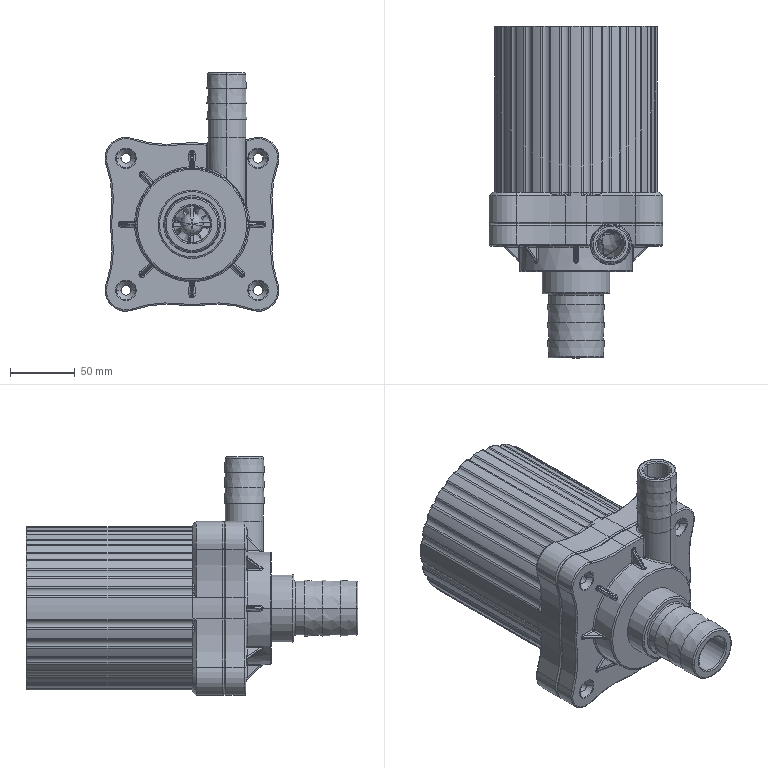Part | SolidWorks | 5 solids | 911 faces | box 134.4 x 256.29 x 184.2 mm | volume 2229611 mm3 | cylinder 312 | torus 227 | spline 190 | plane 91 | sphere 46 | cone 45 | commonest cylinder face diameters 4.2 x68 126 x40 9 x36 2.1 x30 162 x17 7.5 x16